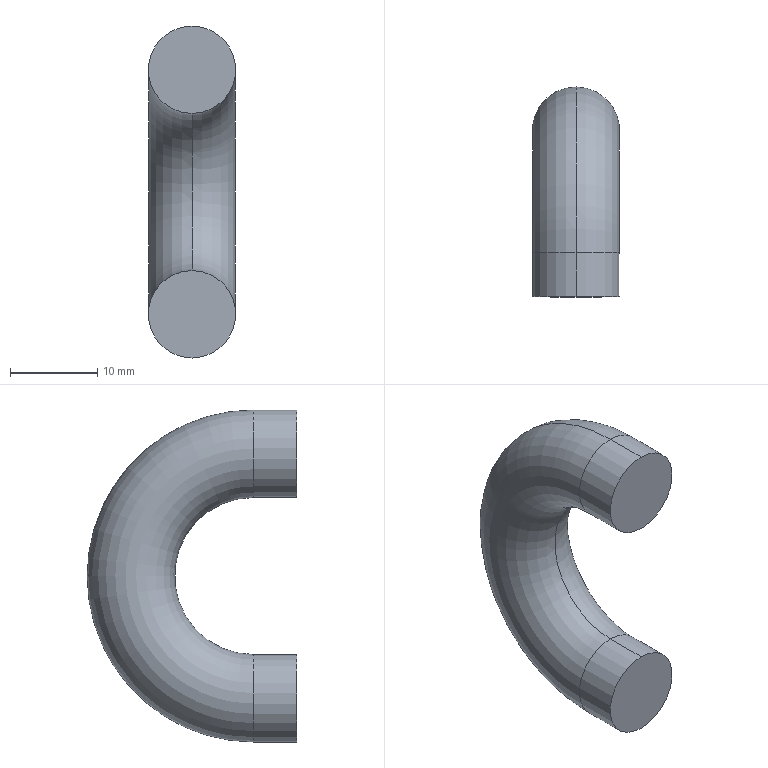Part | STEP file | connecting copper tube 3 | 1 solid | 8 faces | box 10 x 23.975 x 37.95 mm | volume 4234 mm3 | cylinder 4 | torus 2 | plane 2 | commonest cylinder face diameters 10 x4
STEP:
#1=CARTESIAN_POINT('',(0.,0.,0.));
#2=DIRECTION('',(0.,0.,1.));
#3=DIRECTION('',(1.,0.,0.));
#4=AXIS2_PLACEMENT_3D('',#1,#2,#3);
#5=CARTESIAN_POINT('',(0.,5.,5.));
#6=VERTEX_POINT('',#5);
#7=CARTESIAN_POINT('',(0.,5.,-5.));
#8=VERTEX_POINT('',#7);
#9=CARTESIAN_POINT('',(0.,5.,0.));
#10=DIRECTION('',(0.,1.,0.));
#11=DIRECTION('',(0.,0.,1.));
#12=AXIS2_PLACEMENT_3D('',#9,#10,#11);
#13=CIRCLE('',#12,5.);
#14=CARTESIAN_POINT('',(0.,5.,13.975));
#15=DIRECTION('',(1.,0.,0.));
#16=DIRECTION('',(0.,0.,-1.));
#17=AXIS2_PLACEMENT_3D('',#14,#15,#16);
#18=TOROIDAL_SURFACE('',#17,13.975,5.);
#19=CARTESIAN_POINT('',(0.,3.142));
#20=DIRECTION('',(0.,-1.));
#21=VECTOR('',#20,1.);
#22=LINE('',#19,#21);
#23=(GEOMETRIC_REPRESENTATION_CONTEXT(2)PARAMETRIC_REPRESENTATION_CONTEXT()REPRESENTATION_CONTEXT('',''));
#24=DEFINITIONAL_REPRESENTATION('',(#22),#23);
#25=PCURVE('',#18,#24);
#26=CARTESIAN_POINT('',(0.,5.,0.));
#27=DIRECTION('',(0.,-1.,0.));
#28=DIRECTION('',(0.,0.,-1.));
#29=AXIS2_PLACEMENT_3D('',#26,#27,#28);
#30=CYLINDRICAL_SURFACE('',#29,5.);
#31=CARTESIAN_POINT('',(3.142,0.));
#32=DIRECTION('',(-1.,0.));
#33=VECTOR('',#32,1.);
#34=LINE('',#31,#33);
#35=(GEOMETRIC_REPRESENTATION_CONTEXT(2)PARAMETRIC_REPRESENTATION_CONTEXT()REPRESENTATION_CONTEXT('',''));
#36=DEFINITIONAL_REPRESENTATION('',(#34),#35);
#37=PCURVE('',#30,#36);
#38=SURFACE_CURVE('',#13,(#25,#37),.PCURVE_S1.);
#39=EDGE_CURVE('',#6,#8,#38,.T.);
#40=ORIENTED_EDGE('',*,*,#39,.T.);
#41=CARTESIAN_POINT('',(0.,5.,32.95));
#42=VERTEX_POINT('',#41);
#43=CARTESIAN_POINT('',(0.,5.,13.975));
#44=DIRECTION('',(1.,0.,0.));
#45=DIRECTION('',(0.,0.,-1.));
#46=AXIS2_PLACEMENT_3D('',#43,#44,#45);
#47=CIRCLE('',#46,18.975);
#48=CARTESIAN_POINT('',(0.,0.));
#49=DIRECTION('',(1.,0.));
#50=VECTOR('',#49,1.);
#51=LINE('',#48,#50);
#52=(GEOMETRIC_REPRESENTATION_CONTEXT(2)PARAMETRIC_REPRESENTATION_CONTEXT()REPRESENTATION_CONTEXT('',''));
#53=DEFINITIONAL_REPRESENTATION('',(#51),#52);
#54=PCURVE('',#18,#53);
#55=CARTESIAN_POINT('',(0.,5.,13.975));
#56=DIRECTION('',(1.,0.,0.));
#57=DIRECTION('',(0.,0.,-1.));
#58=AXIS2_PLACEMENT_3D('',#55,#56,#57);
#59=TOROIDAL_SURFACE('',#58,13.975,5.);
#60=CARTESIAN_POINT('',(0.,6.283));
#61=DIRECTION('',(1.,0.));
#62=VECTOR('',#61,1.);
#63=LINE('',#60,#62);
#64=(GEOMETRIC_REPRESENTATION_CONTEXT(2)PARAMETRIC_REPRESENTATION_CONTEXT()REPRESENTATION_CONTEXT('',''));
#65=DEFINITIONAL_REPRESENTATION('',(#63),#64);
#66=PCURVE('',#59,#65);
#67=SURFACE_CURVE('',#47,(#54,#66),.PCURVE_S1.);
#68=EDGE_CURVE('',#8,#42,#67,.T.);
#69=ORIENTED_EDGE('',*,*,#68,.T.);
#70=CARTESIAN_POINT('',(0.,5.,22.95));
#71=VERTEX_POINT('',#70);
#72=CARTESIAN_POINT('',(0.,5.,27.95));
#73=DIRECTION('',(0.,-1.,0.));
#74=DIRECTION('',(0.,0.,-1.));
#75=AXIS2_PLACEMENT_3D('',#72,#73,#74);
#76=CIRCLE('',#75,5.);
#77=CARTESIAN_POINT('',(3.142,3.142));
#78=DIRECTION('',(0.,-1.));
#79=VECTOR('',#78,1.);
#80=LINE('',#77,#79);
#81=(GEOMETRIC_REPRESENTATION_CONTEXT(2)PARAMETRIC_REPRESENTATION_CONTEXT()REPRESENTATION_CONTEXT('',''));
#82=DEFINITIONAL_REPRESENTATION('',(#80),#81);
#83=PCURVE('',#18,#82);
#84=CARTESIAN_POINT('',(0.,5.,27.95));
#85=DIRECTION('',(0.,-1.,0.));
#86=DIRECTION('',(0.,0.,-1.));
#87=AXIS2_PLACEMENT_3D('',#84,#85,#86);
#88=CYLINDRICAL_SURFACE('',#87,5.);
#89=CARTESIAN_POINT('',(0.,0.));
#90=DIRECTION('',(1.,0.));
#91=VECTOR('',#90,1.);
#92=LINE('',#89,#91);
#93=(GEOMETRIC_REPRESENTATION_CONTEXT(2)PARAMETRIC_REPRESENTATION_CONTEXT()REPRESENTATION_CONTEXT('',''));
#94=DEFINITIONAL_REPRESENTATION('',(#92),#93);
#95=PCURVE('',#88,#94);
#96=SURFACE_CURVE('',#76,(#83,#95),.PCURVE_S1.);
#97=EDGE_CURVE('',#71,#42,#96,.T.);
#98=ORIENTED_EDGE('',*,*,#97,.F.);
#99=CARTESIAN_POINT('',(0.,5.,13.975));
#100=DIRECTION('',(1.,0.,0.));
#101=DIRECTION('',(0.,0.,-1.));
#102=AXIS2_PLACEMENT_3D('',#99,#100,#101);
#103=CIRCLE('',#102,8.975);
#104=CARTESIAN_POINT('',(0.,3.142));
#105=DIRECTION('',(1.,0.));
#106=VECTOR('',#105,1.);
#107=LINE('',#104,#106);
#108=(GEOMETRIC_REPRESENTATION_CONTEXT(2)PARAMETRIC_REPRESENTATION_CONTEXT()REPRESENTATION_CONTEXT('',''));
#109=DEFINITIONAL_REPRESENTATION('',(#107),#108);
#110=PCURVE('',#18,#109);
#111=CARTESIAN_POINT('',(0.,3.142));
#112=DIRECTION('',(1.,0.));
#113=VECTOR('',#112,1.);
#114=LINE('',#111,#113);
#115=(GEOMETRIC_REPRESENTATION_CONTEXT(2)PARAMETRIC_REPRESENTATION_CONTEXT()REPRESENTATION_CONTEXT('',''));
#116=DEFINITIONAL_REPRESENTATION('',(#114),#115);
#117=PCURVE('',#59,#116);
#118=SURFACE_CURVE('',#103,(#110,#117),.PCURVE_S1.);
#119=EDGE_CURVE('',#6,#71,#118,.T.);
#120=ORIENTED_EDGE('',*,*,#119,.F.);
#121=EDGE_LOOP('',(#40,#69,#98,#120));
#122=FACE_BOUND('',#121,.T.);
#123=ADVANCED_FACE('',(#122),#18,.T.);
#124=ORIENTED_EDGE('',*,*,#39,.F.);
#125=CARTESIAN_POINT('',(0.,0.,5.));
#126=VERTEX_POINT('',#125);
#127=CARTESIAN_POINT('',(0.,5.,5.));
#128=DIRECTION('',(0.,-1.,0.));
#129=VECTOR('',#128,1.);
#130=LINE('',#127,#129);
#131=CARTESIAN_POINT('',(3.142,0.));
#132=DIRECTION('',(0.,1.));
#133=VECTOR('',#132,1.);
#134=LINE('',#131,#133);
#135=(GEOMETRIC_REPRESENTATION_CONTEXT(2)PARAMETRIC_REPRESENTATION_CONTEXT()REPRESENTATION_CONTEXT('',''));
#136=DEFINITIONAL_REPRESENTATION('',(#134),#135);
#137=PCURVE('',#30,#136);
#138=CARTESIAN_POINT('',(0.,5.,0.));
#139=DIRECTION('',(0.,-1.,0.));
#140=DIRECTION('',(0.,0.,-1.));
#141=AXIS2_PLACEMENT_3D('',#138,#139,#140);
#142=CYLINDRICAL_SURFACE('',#141,5.);
#143=CARTESIAN_POINT('',(3.142,0.));
#144=DIRECTION('',(0.,1.));
#145=VECTOR('',#144,1.);
#146=LINE('',#143,#145);
#147=(GEOMETRIC_REPRESENTATION_CONTEXT(2)PARAMETRIC_REPRESENTATION_CONTEXT()REPRESENTATION_CONTEXT('',''));
#148=DEFINITIONAL_REPRESENTATION('',(#146),#147);
#149=PCURVE('',#142,#148);
#150=SURFACE_CURVE('',#130,(#137,#149),.PCURVE_S1.);
#151=EDGE_CURVE('',#6,#126,#150,.T.);
#152=ORIENTED_EDGE('',*,*,#151,.T.);
#153=CARTESIAN_POINT('',(0.,0.,-5.));
#154=VERTEX_POINT('',#153);
#155=CARTESIAN_POINT('',(0.,0.,0.));
#156=DIRECTION('',(0.,1.,0.));
#157=DIRECTION('',(0.,0.,1.));
#158=AXIS2_PLACEMENT_3D('',#155,#156,#157);
#159=CIRCLE('',#158,5.);
#160=CARTESIAN_POINT('',(3.142,5.));
#161=DIRECTION('',(-1.,0.));
#162=VECTOR('',#161,1.);
#163=LINE('',#160,#162);
#164=(GEOMETRIC_REPRESENTATION_CONTEXT(2)PARAMETRIC_REPRESENTATION_CONTEXT()REPRESENTATION_CONTEXT('',''));
#165=DEFINITIONAL_REPRESENTATION('',(#163),#164);
#166=PCURVE('',#30,#165);
#167=CARTESIAN_POINT('',(0.,0.,0.));
#168=DIRECTION('',(0.,1.,0.));
#169=DIRECTION('',(0.,0.,1.));
#170=AXIS2_PLACEMENT_3D('',#167,#168,#169);
#171=PLANE('',#170);
#172=CARTESIAN_POINT('',(0.,0.));
#173=DIRECTION('',(1.,0.));
#174=AXIS2_PLACEMENT_2D('',#172,#173);
#175=CIRCLE('',#174,5.);
#176=(GEOMETRIC_REPRESENTATION_CONTEXT(2)PARAMETRIC_REPRESENTATION_CONTEXT()REPRESENTATION_CONTEXT('',''));
#177=DEFINITIONAL_REPRESENTATION('',(#175),#176);
#178=PCURVE('',#171,#177);
#179=SURFACE_CURVE('',#159,(#166,#178),.PCURVE_S1.);
#180=EDGE_CURVE('',#126,#154,#179,.T.);
#181=ORIENTED_EDGE('',*,*,#180,.T.);
#182=CARTESIAN_POINT('',(0.,5.,-5.));
#183=DIRECTION('',(0.,-1.,0.));
#184=VECTOR('',#183,1.);
#185=LINE('',#182,#184);
#186=CARTESIAN_POINT('',(0.,0.));
#187=DIRECTION('',(0.,1.));
#188=VECTOR('',#187,1.);
#189=LINE('',#186,#188);
#190=(GEOMETRIC_REPRESENTATION_CONTEXT(2)PARAMETRIC_REPRESENTATION_CONTEXT()REPRESENTATION_CONTEXT('',''));
#191=DEFINITIONAL_REPRESENTATION('',(#189),#190);
#192=PCURVE('',#30,#191);
#193=CARTESIAN_POINT('',(6.283,0.));
#194=DIRECTION('',(0.,1.));
#195=VECTOR('',#194,1.);
#196=LINE('',#193,#195);
#197=(GEOMETRIC_REPRESENTATION_CONTEXT(2)PARAMETRIC_REPRESENTATION_CONTEXT()REPRESENTATION_CONTEXT('',''));
#198=DEFINITIONAL_REPRESENTATION('',(#196),#197);
#199=PCURVE('',#142,#198);
#200=SURFACE_CURVE('',#185,(#192,#199),.PCURVE_S1.);
#201=EDGE_CURVE('',#8,#154,#200,.T.);
#202=ORIENTED_EDGE('',*,*,#201,.F.);
#203=EDGE_LOOP('',(#124,#152,#181,#202));
#204=FACE_BOUND('',#203,.T.);
#205=ADVANCED_FACE('',(#204),#30,.T.);
#206=ORIENTED_EDGE('',*,*,#97,.T.);
#207=CARTESIAN_POINT('',(0.,0.,32.95));
#208=VERTEX_POINT('',#207);
#209=CARTESIAN_POINT('',(0.,5.,32.95));
#210=DIRECTION('',(0.,-1.,0.));
#211=VECTOR('',#210,1.);
#212=LINE('',#209,#211);
#213=CARTESIAN_POINT('',(3.142,0.));
#214=DIRECTION('',(0.,1.));
#215=VECTOR('',#214,1.);
#216=LINE('',#213,#215);
#217=(GEOMETRIC_REPRESENTATION_CONTEXT(2)PARAMETRIC_REPRESENTATION_CONTEXT()REPRESENTATION_CONTEXT('',''));
#218=DEFINITIONAL_REPRESENTATION('',(#216),#217);
#219=PCURVE('',#88,#218);
#220=CARTESIAN_POINT('',(0.,5.,27.95));
#221=DIRECTION('',(0.,-1.,0.));
#222=DIRECTION('',(0.,0.,-1.));
#223=AXIS2_PLACEMENT_3D('',#220,#221,#222);
#224=CYLINDRICAL_SURFACE('',#223,5.);
#225=CARTESIAN_POINT('',(3.142,0.));
#226=DIRECTION('',(0.,1.));
#227=VECTOR('',#226,1.);
#228=LINE('',#225,#227);
#229=(GEOMETRIC_REPRESENTATION_CONTEXT(2)PARAMETRIC_REPRESENTATION_CONTEXT()REPRESENTATION_CONTEXT('',''));
#230=DEFINITIONAL_REPRESENTATION('',(#228),#229);
#231=PCURVE('',#224,#230);
#232=SURFACE_CURVE('',#212,(#219,#231),.PCURVE_S1.);
#233=EDGE_CURVE('',#42,#208,#232,.T.);
#234=ORIENTED_EDGE('',*,*,#233,.T.);
#235=CARTESIAN_POINT('',(0.,0.,22.95));
#236=VERTEX_POINT('',#235);
#237=CARTESIAN_POINT('',(0.,0.,27.95));
#238=DIRECTION('',(0.,-1.,0.));
#239=DIRECTION('',(0.,0.,-1.));
#240=AXIS2_PLACEMENT_3D('',#237,#238,#239);
#241=CIRCLE('',#240,5.);
#242=CARTESIAN_POINT('',(0.,5.));
#243=DIRECTION('',(1.,0.));
#244=VECTOR('',#243,1.);
#245=LINE('',#242,#244);
#246=(GEOMETRIC_REPRESENTATION_CONTEXT(2)PARAMETRIC_REPRESENTATION_CONTEXT()REPRESENTATION_CONTEXT('',''));
#247=DEFINITIONAL_REPRESENTATION('',(#245),#246);
#248=PCURVE('',#88,#247);
#249=CARTESIAN_POINT('',(0.,0.,27.95));
#250=DIRECTION('',(0.,-1.,0.));
#251=DIRECTION('',(0.,0.,-1.));
#252=AXIS2_PLACEMENT_3D('',#249,#250,#251);
#253=PLANE('',#252);
#254=CARTESIAN_POINT('',(0.,0.));
#255=DIRECTION('',(1.,0.));
#256=AXIS2_PLACEMENT_2D('',#254,#255);
#257=CIRCLE('',#256,5.);
#258=(GEOMETRIC_REPRESENTATION_CONTEXT(2)PARAMETRIC_REPRESENTATION_CONTEXT()REPRESENTATION_CONTEXT('',''));
#259=DEFINITIONAL_REPRESENTATION('',(#257),#258);
#260=PCURVE('',#253,#259);
#261=SURFACE_CURVE('',#241,(#248,#260),.PCURVE_S1.);
#262=EDGE_CURVE('',#236,#208,#261,.T.);
#263=ORIENTED_EDGE('',*,*,#262,.F.);
#264=CARTESIAN_POINT('',(0.,5.,22.95));
#265=DIRECTION('',(0.,-1.,0.));
#266=VECTOR('',#265,1.);
#267=LINE('',#264,#266);
#268=CARTESIAN_POINT('',(0.,0.));
#269=DIRECTION('',(0.,1.));
#270=VECTOR('',#269,1.);
#271=LINE('',#268,#270);
#272=(GEOMETRIC_REPRESENTATION_CONTEXT(2)PARAMETRIC_REPRESENTATION_CONTEXT()REPRESENTATION_CONTEXT('',''));
#273=DEFINITIONAL_REPRESENTATION('',(#271),#272);
#274=PCURVE('',#88,#273);
#275=CARTESIAN_POINT('',(6.283,0.));
#276=DIRECTION('',(0.,1.));
#277=VECTOR('',#276,1.);
#278=LINE('',#275,#277);
#279=(GEOMETRIC_REPRESENTATION_CONTEXT(2)PARAMETRIC_REPRESENTATION_CONTEXT()REPRESENTATION_CONTEXT('',''));
#280=DEFINITIONAL_REPRESENTATION('',(#278),#279);
#281=PCURVE('',#224,#280);
#282=SURFACE_CURVE('',#267,(#274,#281),.PCURVE_S1.);
#283=EDGE_CURVE('',#71,#236,#282,.T.);
#284=ORIENTED_EDGE('',*,*,#283,.F.);
#285=EDGE_LOOP('',(#206,#234,#263,#284));
#286=FACE_BOUND('',#285,.T.);
#287=ADVANCED_FACE('',(#286),#88,.T.);
#288=ORIENTED_EDGE('',*,*,#233,.F.);
#289=CARTESIAN_POINT('',(0.,5.,27.95));
#290=DIRECTION('',(0.,-1.,0.));
#291=DIRECTION('',(0.,0.,-1.));
#292=AXIS2_PLACEMENT_3D('',#289,#290,#291);
#293=CIRCLE('',#292,5.);
#294=CARTESIAN_POINT('',(0.,0.));
#295=DIRECTION('',(1.,0.));
#296=VECTOR('',#295,1.);
#297=LINE('',#294,#296);
#298=(GEOMETRIC_REPRESENTATION_CONTEXT(2)PARAMETRIC_REPRESENTATION_CONTEXT()REPRESENTATION_CONTEXT('',''));
#299=DEFINITIONAL_REPRESENTATION('',(#297),#298);
#300=PCURVE('',#224,#299);
#301=CARTESIAN_POINT('',(3.142,9.425));
#302=DIRECTION('',(0.,-1.));
#303=VECTOR('',#302,1.);
#304=LINE('',#301,#303);
#305=(GEOMETRIC_REPRESENTATION_CONTEXT(2)PARAMETRIC_REPRESENTATION_CONTEXT()REPRESENTATION_CONTEXT('',''));
#306=DEFINITIONAL_REPRESENTATION('',(#304),#305);
#307=PCURVE('',#59,#306);
#308=SURFACE_CURVE('',#293,(#300,#307),.PCURVE_S1.);
#309=EDGE_CURVE('',#42,#71,#308,.T.);
#310=ORIENTED_EDGE('',*,*,#309,.T.);
#311=ORIENTED_EDGE('',*,*,#283,.T.);
#312=CARTESIAN_POINT('',(0.,0.,27.95));
#313=DIRECTION('',(0.,-1.,0.));
#314=DIRECTION('',(0.,0.,-1.));
#315=AXIS2_PLACEMENT_3D('',#312,#313,#314);
#316=CIRCLE('',#315,5.);
#317=CARTESIAN_POINT('',(0.,5.));
#318=DIRECTION('',(1.,0.));
#319=VECTOR('',#318,1.);
#320=LINE('',#317,#319);
#321=(GEOMETRIC_REPRESENTATION_CONTEXT(2)PARAMETRIC_REPRESENTATION_CONTEXT()REPRESENTATION_CONTEXT('',''));
#322=DEFINITIONAL_REPRESENTATION('',(#320),#321);
#323=PCURVE('',#224,#322);
#324=CARTESIAN_POINT('',(0.,0.));
#325=DIRECTION('',(1.,0.));
#326=AXIS2_PLACEMENT_2D('',#324,#325);
#327=CIRCLE('',#326,5.);
#328=(GEOMETRIC_REPRESENTATION_CONTEXT(2)PARAMETRIC_REPRESENTATION_CONTEXT()REPRESENTATION_CONTEXT('',''));
#329=DEFINITIONAL_REPRESENTATION('',(#327),#328);
#330=PCURVE('',#253,#329);
#331=SURFACE_CURVE('',#316,(#323,#330),.PCURVE_S1.);
#332=EDGE_CURVE('',#208,#236,#331,.T.);
#333=ORIENTED_EDGE('',*,*,#332,.F.);
#334=EDGE_LOOP('',(#288,#310,#311,#333));
#335=FACE_BOUND('',#334,.T.);
#336=ADVANCED_FACE('',(#335),#224,.T.);
#337=ORIENTED_EDGE('',*,*,#68,.F.);
#338=CARTESIAN_POINT('',(0.,5.,0.));
#339=DIRECTION('',(0.,1.,0.));
#340=DIRECTION('',(0.,0.,1.));
#341=AXIS2_PLACEMENT_3D('',#338,#339,#340);
#342=CIRCLE('',#341,5.);
#343=CARTESIAN_POINT('',(0.,9.425));
#344=DIRECTION('',(0.,-1.));
#345=VECTOR('',#344,1.);
#346=LINE('',#343,#345);
#347=(GEOMETRIC_REPRESENTATION_CONTEXT(2)PARAMETRIC_REPRESENTATION_CONTEXT()REPRESENTATION_CONTEXT('',''));
#348=DEFINITIONAL_REPRESENTATION('',(#346),#347);
#349=PCURVE('',#59,#348);
#350=CARTESIAN_POINT('',(9.425,0.));
#351=DIRECTION('',(-1.,0.));
#352=VECTOR('',#351,1.);
#353=LINE('',#350,#352);
#354=(GEOMETRIC_REPRESENTATION_CONTEXT(2)PARAMETRIC_REPRESENTATION_CONTEXT()REPRESENTATION_CONTEXT('',''));
#355=DEFINITIONAL_REPRESENTATION('',(#353),#354);
#356=PCURVE('',#142,#355);
#357=SURFACE_CURVE('',#342,(#349,#356),.PCURVE_S1.);
#358=EDGE_CURVE('',#8,#6,#357,.T.);
#359=ORIENTED_EDGE('',*,*,#358,.T.);
#360=ORIENTED_EDGE('',*,*,#119,.T.);
#361=ORIENTED_EDGE('',*,*,#309,.F.);
#362=EDGE_LOOP('',(#337,#359,#360,#361));
#363=FACE_BOUND('',#362,.T.);
#364=ADVANCED_FACE('',(#363),#59,.T.);
#365=ORIENTED_EDGE('',*,*,#151,.F.);
#366=ORIENTED_EDGE('',*,*,#358,.F.);
#367=ORIENTED_EDGE('',*,*,#201,.T.);
#368=CARTESIAN_POINT('',(0.,0.,0.));
#369=DIRECTION('',(0.,1.,0.));
#370=DIRECTION('',(0.,0.,1.));
#371=AXIS2_PLACEMENT_3D('',#368,#369,#370);
#372=CIRCLE('',#371,5.);
#373=CARTESIAN_POINT('',(9.425,5.));
#374=DIRECTION('',(-1.,0.));
#375=VECTOR('',#374,1.);
#376=LINE('',#373,#375);
#377=(GEOMETRIC_REPRESENTATION_CONTEXT(2)PARAMETRIC_REPRESENTATION_CONTEXT()REPRESENTATION_CONTEXT('',''));
#378=DEFINITIONAL_REPRESENTATION('',(#376),#377);
#379=PCURVE('',#142,#378);
#380=CARTESIAN_POINT('',(0.,0.));
#381=DIRECTION('',(1.,0.));
#382=AXIS2_PLACEMENT_2D('',#380,#381);
#383=CIRCLE('',#382,5.);
#384=(GEOMETRIC_REPRESENTATION_CONTEXT(2)PARAMETRIC_REPRESENTATION_CONTEXT()REPRESENTATION_CONTEXT('',''));
#385=DEFINITIONAL_REPRESENTATION('',(#383),#384);
#386=PCURVE('',#171,#385);
#387=SURFACE_CURVE('',#372,(#379,#386),.PCURVE_S1.);
#388=EDGE_CURVE('',#154,#126,#387,.T.);
#389=ORIENTED_EDGE('',*,*,#388,.T.);
#390=EDGE_LOOP('',(#365,#366,#367,#389));
#391=FACE_BOUND('',#390,.T.);
#392=ADVANCED_FACE('',(#391),#142,.T.);
#393=ORIENTED_EDGE('',*,*,#262,.T.);
#394=ORIENTED_EDGE('',*,*,#332,.T.);
#395=EDGE_LOOP('',(#393,#394));
#396=FACE_BOUND('',#395,.T.);
#397=ADVANCED_FACE('',(#396),#253,.T.);
#398=ORIENTED_EDGE('',*,*,#388,.F.);
#399=ORIENTED_EDGE('',*,*,#180,.F.);
#400=EDGE_LOOP('',(#398,#399));
#401=FACE_BOUND('',#400,.T.);
#402=ADVANCED_FACE('',(#401),#171,.F.);
#403=CLOSED_SHELL('',(#123,#205,#287,#336,#364,#392,#397,#402));
#404=MANIFOLD_SOLID_BREP('',#403);
#405=(LENGTH_UNIT()NAMED_UNIT(*)SI_UNIT(.MILLI.,.METRE.));
#406=UNCERTAINTY_MEASURE_WITH_UNIT(LENGTH_MEASURE(0.0000001),#405,'','');
#407=(NAMED_UNIT(*)PLANE_ANGLE_UNIT()SI_UNIT($,.RADIAN.));
#408=(NAMED_UNIT(*)SI_UNIT($,.STERADIAN.)SOLID_ANGLE_UNIT());
#409=(GEOMETRIC_REPRESENTATION_CONTEXT(3)GLOBAL_UNCERTAINTY_ASSIGNED_CONTEXT((#406))GLOBAL_UNIT_ASSIGNED_CONTEXT((#405,#407,#408))REPRESENTATION_CONTEXT('',''));
#410=ADVANCED_BREP_SHAPE_REPRESENTATION('',(#4,#404),#409);